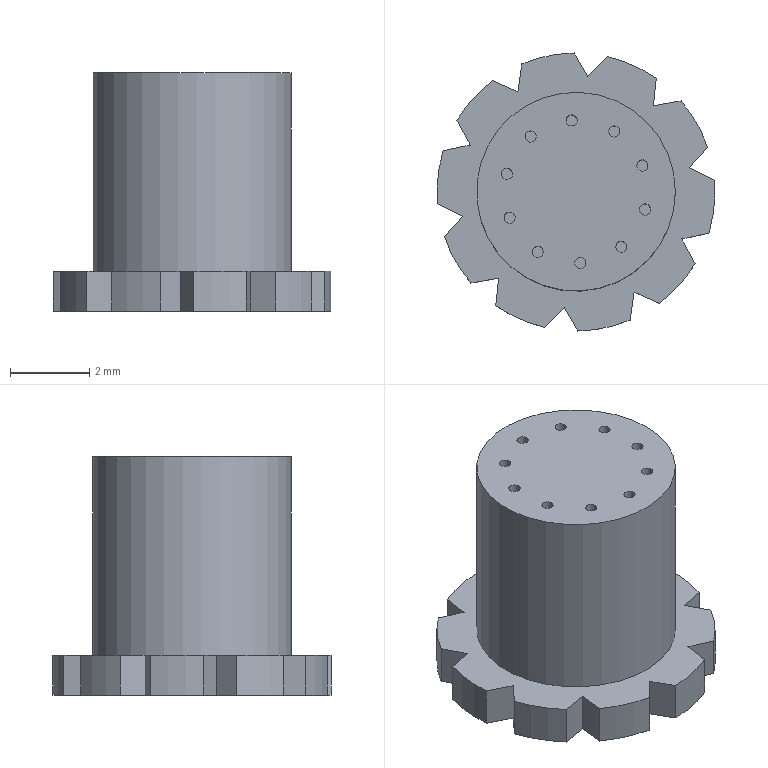Part | NX | features DATUM_CSYS 3, CYLINDER 2, EXTRUDE 2, SKETCH 2 | 1 solid | 54 faces | box 7 x 6.999 x 6 mm | volume 131.027 mm3 | plane 33 | cylinder 21 | commonest cylinder face diameters 0.283 x10 7 x10 5 x1
STEP:
#1=CARTESIAN_POINT('',(-0.7918,-3.409,0.));
#2=VERTEX_POINT('',#1);
#3=CARTESIAN_POINT('',(-0.7918,-3.409,-1.));
#4=VERTEX_POINT('',#3);
#5=CARTESIAN_POINT('',(-0.7918,-3.409,0.));
#6=DIRECTION('',(0.,0.,-1.));
#7=VECTOR('',#6,1000.);
#8=LINE('',#5,#7);
#9=EDGE_CURVE('',#2,#4,#8,.T.);
#10=ORIENTED_EDGE('',*,*,#9,.F.);
#11=CARTESIAN_POINT('',(-2.021,-2.858,0.));
#12=VERTEX_POINT('',#11);
#13=CARTESIAN_POINT('',(0.,0.,0.));
#14=DIRECTION('',(0.,0.,-1.));
#15=DIRECTION('',(1.,0.,0.));
#16=AXIS2_PLACEMENT_3D('',#13,#14,#15);
#17=CIRCLE('',#16,3.5);
#18=EDGE_CURVE('',#2,#12,#17,.T.);
#19=ORIENTED_EDGE('',*,*,#18,.T.);
#20=CARTESIAN_POINT('',(-2.021,-2.858,-1.));
#21=VERTEX_POINT('',#20);
#22=CARTESIAN_POINT('',(-2.021,-2.858,0.));
#23=DIRECTION('',(0.,0.,-1.));
#24=VECTOR('',#23,1000.);
#25=LINE('',#22,#24);
#26=EDGE_CURVE('',#21,#12,#25,.F.);
#27=ORIENTED_EDGE('',*,*,#26,.F.);
#28=CARTESIAN_POINT('',(0.,0.,-1.));
#29=DIRECTION('',(0.,0.,1.));
#30=DIRECTION('',(1.,0.,0.));
#31=AXIS2_PLACEMENT_3D('',#28,#29,#30);
#32=CIRCLE('',#31,3.5);
#33=EDGE_CURVE('',#21,#4,#32,.T.);
#34=ORIENTED_EDGE('',*,*,#33,.T.);
#35=EDGE_LOOP('',(#10,#19,#27,#34));
#36=FACE_BOUND('',#35,.T.);
#37=CARTESIAN_POINT('',(0.,0.,0.));
#38=DIRECTION('',(0.,0.,-1.));
#39=DIRECTION('',(1.,0.,0.));
#40=AXIS2_PLACEMENT_3D('',#37,#38,#39);
#41=CYLINDRICAL_SURFACE('',#40,3.5);
#42=ADVANCED_FACE('',(#36),#41,.T.);
#43=CARTESIAN_POINT('',(-2.093,2.805,-1.));
#44=VERTEX_POINT('',#43);
#45=CARTESIAN_POINT('',(-2.093,2.805,0.));
#46=VERTEX_POINT('',#45);
#47=CARTESIAN_POINT('',(-2.093,2.805,0.));
#48=DIRECTION('',(0.,0.,-1.));
#49=VECTOR('',#48,1000.);
#50=LINE('',#47,#49);
#51=EDGE_CURVE('',#44,#46,#50,.F.);
#52=ORIENTED_EDGE('',*,*,#51,.F.);
#53=CARTESIAN_POINT('',(-2.998,1.807,-1.));
#54=VERTEX_POINT('',#53);
#55=CARTESIAN_POINT('',(0.,0.,-1.));
#56=DIRECTION('',(0.,0.,1.));
#57=DIRECTION('',(1.,0.,0.));
#58=AXIS2_PLACEMENT_3D('',#55,#56,#57);
#59=CIRCLE('',#58,3.5);
#60=EDGE_CURVE('',#44,#54,#59,.T.);
#61=ORIENTED_EDGE('',*,*,#60,.T.);
#62=CARTESIAN_POINT('',(-2.998,1.807,0.));
#63=VERTEX_POINT('',#62);
#64=CARTESIAN_POINT('',(-2.998,1.807,0.));
#65=DIRECTION('',(0.,0.,-1.));
#66=VECTOR('',#65,1000.);
#67=LINE('',#64,#66);
#68=EDGE_CURVE('',#63,#54,#67,.T.);
#69=ORIENTED_EDGE('',*,*,#68,.F.);
#70=CARTESIAN_POINT('',(0.,0.,0.));
#71=DIRECTION('',(0.,0.,-1.));
#72=DIRECTION('',(1.,0.,0.));
#73=AXIS2_PLACEMENT_3D('',#70,#71,#72);
#74=CIRCLE('',#73,3.5);
#75=EDGE_CURVE('',#63,#46,#74,.T.);
#76=ORIENTED_EDGE('',*,*,#75,.T.);
#77=EDGE_LOOP('',(#52,#61,#69,#76));
#78=FACE_BOUND('',#77,.T.);
#79=CARTESIAN_POINT('',(0.,0.,0.));
#80=DIRECTION('',(0.,0.,-1.));
#81=DIRECTION('',(1.,0.,0.));
#82=AXIS2_PLACEMENT_3D('',#79,#80,#81);
#83=CYLINDRICAL_SURFACE('',#82,3.5);
#84=ADVANCED_FACE('',(#78),#83,.T.);
#85=CARTESIAN_POINT('',(0.04482,-3.5,-1.));
#86=VERTEX_POINT('',#85);
#87=CARTESIAN_POINT('',(0.04482,-3.5,0.));
#88=VERTEX_POINT('',#87);
#89=CARTESIAN_POINT('',(0.04482,-3.5,0.));
#90=DIRECTION('',(0.,0.,-1.));
#91=VECTOR('',#90,1000.);
#92=LINE('',#89,#91);
#93=EDGE_CURVE('',#86,#88,#92,.F.);
#94=ORIENTED_EDGE('',*,*,#93,.F.);
#95=CARTESIAN_POINT('',(1.363,-3.224,-1.));
#96=VERTEX_POINT('',#95);
#97=CARTESIAN_POINT('',(0.,0.,-1.));
#98=DIRECTION('',(0.,0.,1.));
#99=DIRECTION('',(1.,0.,0.));
#100=AXIS2_PLACEMENT_3D('',#97,#98,#99);
#101=CIRCLE('',#100,3.5);
#102=EDGE_CURVE('',#86,#96,#101,.T.);
#103=ORIENTED_EDGE('',*,*,#102,.T.);
#104=CARTESIAN_POINT('',(1.363,-3.224,0.));
#105=VERTEX_POINT('',#104);
#106=CARTESIAN_POINT('',(1.363,-3.224,0.));
#107=DIRECTION('',(0.,0.,-1.));
#108=VECTOR('',#107,1000.);
#109=LINE('',#106,#108);
#110=EDGE_CURVE('',#105,#96,#109,.T.);
#111=ORIENTED_EDGE('',*,*,#110,.F.);
#112=CARTESIAN_POINT('',(0.,0.,0.));
#113=DIRECTION('',(0.,0.,-1.));
#114=DIRECTION('',(1.,0.,0.));
#115=AXIS2_PLACEMENT_3D('',#112,#113,#114);
#116=CIRCLE('',#115,3.5);
#117=EDGE_CURVE('',#105,#88,#116,.T.);
#118=ORIENTED_EDGE('',*,*,#117,.T.);
#119=EDGE_LOOP('',(#94,#103,#111,#118));
#120=FACE_BOUND('',#119,.T.);
#121=CARTESIAN_POINT('',(0.,0.,0.));
#122=DIRECTION('',(0.,0.,-1.));
#123=DIRECTION('',(1.,0.,0.));
#124=AXIS2_PLACEMENT_3D('',#121,#122,#123);
#125=CYLINDRICAL_SURFACE('',#124,3.5);
#126=ADVANCED_FACE('',(#120),#125,.T.);
#127=CARTESIAN_POINT('',(-2.644,-2.293,0.));
#128=VERTEX_POINT('',#127);
#129=CARTESIAN_POINT('',(-2.644,-2.293,-1.));
#130=VERTEX_POINT('',#129);
#131=CARTESIAN_POINT('',(-2.644,-2.293,0.));
#132=DIRECTION('',(0.,0.,-1.));
#133=VECTOR('',#132,1000.);
#134=LINE('',#131,#133);
#135=EDGE_CURVE('',#128,#130,#134,.T.);
#136=ORIENTED_EDGE('',*,*,#135,.F.);
#137=CARTESIAN_POINT('',(-3.315,-1.124,0.));
#138=VERTEX_POINT('',#137);
#139=CARTESIAN_POINT('',(0.,0.,0.));
#140=DIRECTION('',(0.,0.,-1.));
#141=DIRECTION('',(1.,0.,0.));
#142=AXIS2_PLACEMENT_3D('',#139,#140,#141);
#143=CIRCLE('',#142,3.5);
#144=EDGE_CURVE('',#128,#138,#143,.T.);
#145=ORIENTED_EDGE('',*,*,#144,.T.);
#146=CARTESIAN_POINT('',(-3.315,-1.124,-1.));
#147=VERTEX_POINT('',#146);
#148=CARTESIAN_POINT('',(-3.315,-1.124,0.));
#149=DIRECTION('',(0.,0.,-1.));
#150=VECTOR('',#149,1000.);
#151=LINE('',#148,#150);
#152=EDGE_CURVE('',#147,#138,#151,.F.);
#153=ORIENTED_EDGE('',*,*,#152,.F.);
#154=CARTESIAN_POINT('',(0.,0.,-1.));
#155=DIRECTION('',(0.,0.,1.));
#156=DIRECTION('',(1.,0.,0.));
#157=AXIS2_PLACEMENT_3D('',#154,#155,#156);
#158=CIRCLE('',#157,3.5);
#159=EDGE_CURVE('',#147,#130,#158,.T.);
#160=ORIENTED_EDGE('',*,*,#159,.T.);
#161=EDGE_LOOP('',(#136,#145,#153,#160));
#162=FACE_BOUND('',#161,.T.);
#163=CARTESIAN_POINT('',(0.,0.,0.));
#164=DIRECTION('',(0.,0.,-1.));
#165=DIRECTION('',(1.,0.,0.));
#166=AXIS2_PLACEMENT_3D('',#163,#164,#165);
#167=CYLINDRICAL_SURFACE('',#166,3.5);
#168=ADVANCED_FACE('',(#162),#167,.T.);
#169=CARTESIAN_POINT('',(2.998,-1.807,0.));
#170=VERTEX_POINT('',#169);
#171=CARTESIAN_POINT('',(2.998,-1.807,-1.));
#172=VERTEX_POINT('',#171);
#173=CARTESIAN_POINT('',(2.998,-1.807,0.));
#174=DIRECTION('',(0.,0.,-1.));
#175=VECTOR('',#174,1000.);
#176=LINE('',#173,#175);
#177=EDGE_CURVE('',#170,#172,#176,.T.);
#178=ORIENTED_EDGE('',*,*,#177,.F.);
#179=CARTESIAN_POINT('',(2.093,-2.805,0.));
#180=VERTEX_POINT('',#179);
#181=CARTESIAN_POINT('',(0.,0.,0.));
#182=DIRECTION('',(0.,0.,-1.));
#183=DIRECTION('',(1.,0.,0.));
#184=AXIS2_PLACEMENT_3D('',#181,#182,#183);
#185=CIRCLE('',#184,3.5);
#186=EDGE_CURVE('',#170,#180,#185,.T.);
#187=ORIENTED_EDGE('',*,*,#186,.T.);
#188=CARTESIAN_POINT('',(2.093,-2.805,-1.));
#189=VERTEX_POINT('',#188);
#190=CARTESIAN_POINT('',(2.093,-2.805,0.));
#191=DIRECTION('',(0.,0.,-1.));
#192=VECTOR('',#191,1000.);
#193=LINE('',#190,#192);
#194=EDGE_CURVE('',#189,#180,#193,.F.);
#195=ORIENTED_EDGE('',*,*,#194,.F.);
#196=CARTESIAN_POINT('',(0.,0.,-1.));
#197=DIRECTION('',(0.,0.,1.));
#198=DIRECTION('',(1.,0.,0.));
#199=AXIS2_PLACEMENT_3D('',#196,#197,#198);
#200=CIRCLE('',#199,3.5);
#201=EDGE_CURVE('',#189,#172,#200,.T.);
#202=ORIENTED_EDGE('',*,*,#201,.T.);
#203=EDGE_LOOP('',(#178,#187,#195,#202));
#204=FACE_BOUND('',#203,.T.);
#205=CARTESIAN_POINT('',(0.,0.,0.));
#206=DIRECTION('',(0.,0.,-1.));
#207=DIRECTION('',(1.,0.,0.));
#208=AXIS2_PLACEMENT_3D('',#205,#206,#207);
#209=CYLINDRICAL_SURFACE('',#208,3.5);
#210=ADVANCED_FACE('',(#204),#209,.T.);
#211=CARTESIAN_POINT('',(2.021,2.858,-1.));
#212=VERTEX_POINT('',#211);
#213=CARTESIAN_POINT('',(2.021,2.858,0.));
#214=VERTEX_POINT('',#213);
#215=CARTESIAN_POINT('',(2.021,2.858,0.));
#216=DIRECTION('',(0.,0.,-1.));
#217=VECTOR('',#216,1000.);
#218=LINE('',#215,#217);
#219=EDGE_CURVE('',#212,#214,#218,.F.);
#220=ORIENTED_EDGE('',*,*,#219,.F.);
#221=CARTESIAN_POINT('',(0.7918,3.409,-1.));
#222=VERTEX_POINT('',#221);
#223=CARTESIAN_POINT('',(0.,0.,-1.));
#224=DIRECTION('',(0.,0.,1.));
#225=DIRECTION('',(1.,0.,0.));
#226=AXIS2_PLACEMENT_3D('',#223,#224,#225);
#227=CIRCLE('',#226,3.5);
#228=EDGE_CURVE('',#212,#222,#227,.T.);
#229=ORIENTED_EDGE('',*,*,#228,.T.);
#230=CARTESIAN_POINT('',(0.7918,3.409,0.));
#231=VERTEX_POINT('',#230);
#232=CARTESIAN_POINT('',(0.7918,3.409,0.));
#233=DIRECTION('',(0.,0.,-1.));
#234=VECTOR('',#233,1000.);
#235=LINE('',#232,#234);
#236=EDGE_CURVE('',#231,#222,#235,.T.);
#237=ORIENTED_EDGE('',*,*,#236,.F.);
#238=CARTESIAN_POINT('',(0.,0.,0.));
#239=DIRECTION('',(0.,0.,-1.));
#240=DIRECTION('',(1.,0.,0.));
#241=AXIS2_PLACEMENT_3D('',#238,#239,#240);
#242=CIRCLE('',#241,3.5);
#243=EDGE_CURVE('',#231,#214,#242,.T.);
#244=ORIENTED_EDGE('',*,*,#243,.T.);
#245=EDGE_LOOP('',(#220,#229,#237,#244));
#246=FACE_BOUND('',#245,.T.);
#247=CARTESIAN_POINT('',(0.,0.,0.));
#248=DIRECTION('',(0.,0.,-1.));
#249=DIRECTION('',(1.,0.,0.));
#250=AXIS2_PLACEMENT_3D('',#247,#248,#249);
#251=CYLINDRICAL_SURFACE('',#250,3.5);
#252=ADVANCED_FACE('',(#246),#251,.T.);
#253=CARTESIAN_POINT('',(-3.487,-0.3005,0.));
#254=VERTEX_POINT('',#253);
#255=CARTESIAN_POINT('',(-3.487,-0.3005,-1.));
#256=VERTEX_POINT('',#255);
#257=CARTESIAN_POINT('',(-3.487,-0.3005,0.));
#258=DIRECTION('',(0.,0.,-1.));
#259=VECTOR('',#258,1000.);
#260=LINE('',#257,#259);
#261=EDGE_CURVE('',#254,#256,#260,.T.);
#262=ORIENTED_EDGE('',*,*,#261,.F.);
#263=CARTESIAN_POINT('',(-3.342,1.039,0.));
#264=VERTEX_POINT('',#263);
#265=CARTESIAN_POINT('',(0.,0.,0.));
#266=DIRECTION('',(0.,0.,-1.));
#267=DIRECTION('',(1.,0.,0.));
#268=AXIS2_PLACEMENT_3D('',#265,#266,#267);
#269=CIRCLE('',#268,3.5);
#270=EDGE_CURVE('',#254,#264,#269,.T.);
#271=ORIENTED_EDGE('',*,*,#270,.T.);
#272=CARTESIAN_POINT('',(-3.342,1.039,-1.));
#273=VERTEX_POINT('',#272);
#274=CARTESIAN_POINT('',(-3.342,1.039,0.));
#275=DIRECTION('',(0.,0.,-1.));
#276=VECTOR('',#275,1000.);
#277=LINE('',#274,#276);
#278=EDGE_CURVE('',#273,#264,#277,.F.);
#279=ORIENTED_EDGE('',*,*,#278,.F.);
#280=CARTESIAN_POINT('',(0.,0.,-1.));
#281=DIRECTION('',(0.,0.,1.));
#282=DIRECTION('',(1.,0.,0.));
#283=AXIS2_PLACEMENT_3D('',#280,#281,#282);
#284=CIRCLE('',#283,3.5);
#285=EDGE_CURVE('',#273,#256,#284,.T.);
#286=ORIENTED_EDGE('',*,*,#285,.T.);
#287=EDGE_LOOP('',(#262,#271,#279,#286));
#288=FACE_BOUND('',#287,.T.);
#289=CARTESIAN_POINT('',(0.,0.,0.));
#290=DIRECTION('',(0.,0.,-1.));
#291=DIRECTION('',(1.,0.,0.));
#292=AXIS2_PLACEMENT_3D('',#289,#290,#291);
#293=CYLINDRICAL_SURFACE('',#292,3.5);
#294=ADVANCED_FACE('',(#288),#293,.T.);
#295=CARTESIAN_POINT('',(-1.363,3.224,0.));
#296=VERTEX_POINT('',#295);
#297=CARTESIAN_POINT('',(-1.363,3.224,-1.));
#298=VERTEX_POINT('',#297);
#299=CARTESIAN_POINT('',(-1.363,3.224,0.));
#300=DIRECTION('',(0.,0.,-1.));
#301=VECTOR('',#300,1000.);
#302=LINE('',#299,#301);
#303=EDGE_CURVE('',#296,#298,#302,.T.);
#304=ORIENTED_EDGE('',*,*,#303,.F.);
#305=CARTESIAN_POINT('',(-0.04482,3.5,0.));
#306=VERTEX_POINT('',#305);
#307=CARTESIAN_POINT('',(0.,0.,0.));
#308=DIRECTION('',(0.,0.,-1.));
#309=DIRECTION('',(1.,0.,0.));
#310=AXIS2_PLACEMENT_3D('',#307,#308,#309);
#311=CIRCLE('',#310,3.5);
#312=EDGE_CURVE('',#296,#306,#311,.T.);
#313=ORIENTED_EDGE('',*,*,#312,.T.);
#314=CARTESIAN_POINT('',(-0.04482,3.5,-1.));
#315=VERTEX_POINT('',#314);
#316=CARTESIAN_POINT('',(-0.04482,3.5,0.));
#317=DIRECTION('',(0.,0.,-1.));
#318=VECTOR('',#317,1000.);
#319=LINE('',#316,#318);
#320=EDGE_CURVE('',#315,#306,#319,.F.);
#321=ORIENTED_EDGE('',*,*,#320,.F.);
#322=CARTESIAN_POINT('',(0.,0.,-1.));
#323=DIRECTION('',(0.,0.,1.));
#324=DIRECTION('',(1.,0.,0.));
#325=AXIS2_PLACEMENT_3D('',#322,#323,#324);
#326=CIRCLE('',#325,3.5);
#327=EDGE_CURVE('',#315,#298,#326,.T.);
#328=ORIENTED_EDGE('',*,*,#327,.T.);
#329=EDGE_LOOP('',(#304,#313,#321,#328));
#330=FACE_BOUND('',#329,.T.);
#331=CARTESIAN_POINT('',(0.,0.,0.));
#332=DIRECTION('',(0.,0.,-1.));
#333=DIRECTION('',(1.,0.,0.));
#334=AXIS2_PLACEMENT_3D('',#331,#332,#333);
#335=CYLINDRICAL_SURFACE('',#334,3.5);
#336=ADVANCED_FACE('',(#330),#335,.T.);
#337=CARTESIAN_POINT('',(3.342,-1.039,-1.));
#338=VERTEX_POINT('',#337);
#339=CARTESIAN_POINT('',(3.342,-1.039,0.));
#340=VERTEX_POINT('',#339);
#341=CARTESIAN_POINT('',(3.342,-1.039,0.));
#342=DIRECTION('',(0.,0.,-1.));
#343=VECTOR('',#342,1000.);
#344=LINE('',#341,#343);
#345=EDGE_CURVE('',#338,#340,#344,.F.);
#346=ORIENTED_EDGE('',*,*,#345,.F.);
#347=CARTESIAN_POINT('',(3.487,0.3005,-1.));
#348=VERTEX_POINT('',#347);
#349=CARTESIAN_POINT('',(0.,0.,-1.));
#350=DIRECTION('',(0.,0.,1.));
#351=DIRECTION('',(1.,0.,0.));
#352=AXIS2_PLACEMENT_3D('',#349,#350,#351);
#353=CIRCLE('',#352,3.5);
#354=EDGE_CURVE('',#338,#348,#353,.T.);
#355=ORIENTED_EDGE('',*,*,#354,.T.);
#356=CARTESIAN_POINT('',(3.487,0.3005,0.));
#357=VERTEX_POINT('',#356);
#358=CARTESIAN_POINT('',(3.487,0.3005,0.));
#359=DIRECTION('',(0.,0.,-1.));
#360=VECTOR('',#359,1000.);
#361=LINE('',#358,#360);
#362=EDGE_CURVE('',#357,#348,#361,.T.);
#363=ORIENTED_EDGE('',*,*,#362,.F.);
#364=CARTESIAN_POINT('',(0.,0.,0.));
#365=DIRECTION('',(0.,0.,-1.));
#366=DIRECTION('',(1.,0.,0.));
#367=AXIS2_PLACEMENT_3D('',#364,#365,#366);
#368=CIRCLE('',#367,3.5);
#369=EDGE_CURVE('',#357,#340,#368,.T.);
#370=ORIENTED_EDGE('',*,*,#369,.T.);
#371=EDGE_LOOP('',(#346,#355,#363,#370));
#372=FACE_BOUND('',#371,.T.);
#373=CARTESIAN_POINT('',(0.,0.,0.));
#374=DIRECTION('',(0.,0.,-1.));
#375=DIRECTION('',(1.,0.,0.));
#376=AXIS2_PLACEMENT_3D('',#373,#374,#375);
#377=CYLINDRICAL_SURFACE('',#376,3.5);
#378=ADVANCED_FACE('',(#372),#377,.T.);
#379=CARTESIAN_POINT('',(0.03282,1.793,5.));
#380=VERTEX_POINT('',#379);
#381=CARTESIAN_POINT('',(-0.1085,1.793,5.));
#382=DIRECTION('',(0.,0.,1.));
#383=DIRECTION('',(1.,0.,0.));
#384=AXIS2_PLACEMENT_3D('',#381,#382,#383);
#385=CIRCLE('',#384,0.1413);
#386=EDGE_CURVE('',#380,#380,#385,.T.);
#387=ORIENTED_EDGE('',*,*,#386,.F.);
#388=EDGE_LOOP('',(#387));
#389=FACE_BOUND('',#388,.T.);
#390=CARTESIAN_POINT('',(-1.08,-1.431,5.));
#391=VERTEX_POINT('',#390);
#392=CARTESIAN_POINT('',(-0.9659,-1.514,5.));
#393=DIRECTION('',(0.,0.,1.));
#394=DIRECTION('',(-0.809,0.5878,0.));
#395=AXIS2_PLACEMENT_3D('',#392,#393,#394);
#396=CIRCLE('',#395,0.1413);
#397=EDGE_CURVE('',#391,#391,#396,.T.);
#398=ORIENTED_EDGE('',*,*,#397,.F.);
#399=EDGE_LOOP('',(#398));
#400=FACE_BOUND('',#399,.T.);
#401=CARTESIAN_POINT('',(-1.027,1.47,5.));
#402=VERTEX_POINT('',#401);
#403=CARTESIAN_POINT('',(-1.141,1.386,5.));
#404=DIRECTION('',(0.,0.,1.));
#405=DIRECTION('',(0.809,0.5878,0.));
#406=AXIS2_PLACEMENT_3D('',#403,#404,#405);
#407=CIRCLE('',#406,0.1413);
#408=EDGE_CURVE('',#402,#402,#407,.T.);
#409=ORIENTED_EDGE('',*,*,#408,.F.);
#410=EDGE_LOOP('',(#409));
#411=FACE_BOUND('',#410,.T.);
#412=CARTESIAN_POINT('',(-1.715,-0.5227,5.));
#413=VERTEX_POINT('',#412);
#414=CARTESIAN_POINT('',(-1.671,-0.6571,5.));
#415=DIRECTION('',(0.,0.,1.));
#416=DIRECTION('',(-0.309,0.9511,0.));
#417=AXIS2_PLACEMENT_3D('',#414,#415,#416);
#418=CIRCLE('',#417,0.1413);
#419=EDGE_CURVE('',#413,#413,#418,.T.);
#420=ORIENTED_EDGE('',*,*,#419,.F.);
#421=EDGE_LOOP('',(#420));
#422=FACE_BOUND('',#421,.T.);
#423=CARTESIAN_POINT('',(1.715,0.5227,5.));
#424=VERTEX_POINT('',#423);
#425=CARTESIAN_POINT('',(1.671,0.6571,5.));
#426=DIRECTION('',(0.,0.,1.));
#427=DIRECTION('',(0.309,-0.9511,0.));
#428=AXIS2_PLACEMENT_3D('',#425,#426,#427);
#429=CIRCLE('',#428,0.1413);
#430=EDGE_CURVE('',#424,#424,#429,.T.);
#431=ORIENTED_EDGE('',*,*,#430,.F.);
#432=EDGE_LOOP('',(#431));
#433=FACE_BOUND('',#432,.T.);
#434=CARTESIAN_POINT('',(1.027,-1.47,5.));
#435=VERTEX_POINT('',#434);
#436=CARTESIAN_POINT('',(1.141,-1.386,5.));
#437=DIRECTION('',(0.,0.,1.));
#438=DIRECTION('',(-0.809,-0.5878,0.));
#439=AXIS2_PLACEMENT_3D('',#436,#437,#438);
#440=CIRCLE('',#439,0.1413);
#441=EDGE_CURVE('',#435,#435,#440,.T.);
#442=ORIENTED_EDGE('',*,*,#441,.F.);
#443=EDGE_LOOP('',(#442));
#444=FACE_BOUND('',#443,.T.);
#445=CARTESIAN_POINT('',(1.08,1.431,5.));
#446=VERTEX_POINT('',#445);
#447=CARTESIAN_POINT('',(0.9659,1.514,5.));
#448=DIRECTION('',(0.,0.,1.));
#449=DIRECTION('',(0.809,-0.5878,0.));
#450=AXIS2_PLACEMENT_3D('',#447,#448,#449);
#451=CIRCLE('',#450,0.1413);
#452=EDGE_CURVE('',#446,#446,#451,.T.);
#453=ORIENTED_EDGE('',*,*,#452,.F.);
#454=EDGE_LOOP('',(#453));
#455=FACE_BOUND('',#454,.T.);
#456=CARTESIAN_POINT('',(-0.03282,-1.793,5.));
#457=VERTEX_POINT('',#456);
#458=CARTESIAN_POINT('',(0.1085,-1.793,5.));
#459=DIRECTION('',(0.,0.,1.));
#460=DIRECTION('',(-1.,0.,0.));
#461=AXIS2_PLACEMENT_3D('',#458,#459,#460);
#462=CIRCLE('',#461,0.1413);
#463=EDGE_CURVE('',#457,#457,#462,.T.);
#464=ORIENTED_EDGE('',*,*,#463,.F.);
#465=EDGE_LOOP('',(#464));
#466=FACE_BOUND('',#465,.T.);
#467=CARTESIAN_POINT('',(-1.695,0.5852,5.));
#468=VERTEX_POINT('',#467);
#469=CARTESIAN_POINT('',(-1.738,0.4508,5.));
#470=DIRECTION('',(0.,0.,1.));
#471=DIRECTION('',(0.309,0.9511,0.));
#472=AXIS2_PLACEMENT_3D('',#469,#470,#471);
#473=CIRCLE('',#472,0.1413);
#474=EDGE_CURVE('',#468,#468,#473,.T.);
#475=ORIENTED_EDGE('',*,*,#474,.F.);
#476=EDGE_LOOP('',(#475));
#477=FACE_BOUND('',#476,.T.);
#478=CARTESIAN_POINT('',(1.695,-0.5852,5.));
#479=VERTEX_POINT('',#478);
#480=CARTESIAN_POINT('',(1.738,-0.4508,5.));
#481=DIRECTION('',(0.,0.,1.));
#482=DIRECTION('',(-0.309,-0.9511,0.));
#483=AXIS2_PLACEMENT_3D('',#480,#481,#482);
#484=CIRCLE('',#483,0.1413);
#485=EDGE_CURVE('',#479,#479,#484,.T.);
#486=ORIENTED_EDGE('',*,*,#485,.F.);
#487=EDGE_LOOP('',(#486));
#488=FACE_BOUND('',#487,.T.);
#489=CARTESIAN_POINT('',(2.5,0.,5.));
#490=VERTEX_POINT('',#489);
#491=CARTESIAN_POINT('',(0.,0.,5.));
#492=DIRECTION('',(0.,0.,-1.));
#493=DIRECTION('',(1.,0.,0.));
#494=AXIS2_PLACEMENT_3D('',#491,#492,#493);
#495=CIRCLE('',#494,2.5);
#496=EDGE_CURVE('',#490,#490,#495,.T.);
#497=ORIENTED_EDGE('',*,*,#496,.F.);
#498=EDGE_LOOP('',(#497));
#499=FACE_BOUND('',#498,.T.);
#500=CARTESIAN_POINT('',(0.,0.,5.));
#501=DIRECTION('',(0.,0.,1.));
#502=DIRECTION('',(1.,0.,0.));
#503=AXIS2_PLACEMENT_3D('',#500,#501,#502);
#504=PLANE('',#503);
#505=ADVANCED_FACE('',(#389,#400,#411,#422,#433,#444,#455,#466,#477,#488,#499),#504,.T.);
#506=ORIENTED_EDGE('',*,*,#496,.T.);
#507=EDGE_LOOP('',(#506));
#508=FACE_BOUND('',#507,.T.);
#509=CARTESIAN_POINT('',(2.5,0.,0.));
#510=VERTEX_POINT('',#509);
#511=CARTESIAN_POINT('',(0.,0.,0.));
#512=DIRECTION('',(0.,0.,1.));
#513=DIRECTION('',(1.,0.,0.));
#514=AXIS2_PLACEMENT_3D('',#511,#512,#513);
#515=CIRCLE('',#514,2.5);
#516=EDGE_CURVE('',#510,#510,#515,.T.);
#517=ORIENTED_EDGE('',*,*,#516,.T.);
#518=EDGE_LOOP('',(#517));
#519=FACE_BOUND('',#518,.T.);
#520=CARTESIAN_POINT('',(0.,0.,0.));
#521=DIRECTION('',(0.,0.,1.));
#522=DIRECTION('',(1.,0.,0.));
#523=AXIS2_PLACEMENT_3D('',#520,#521,#522);
#524=CYLINDRICAL_SURFACE('',#523,2.5);
#525=ADVANCED_FACE('',(#508,#519),#524,.T.);
#526=ORIENTED_EDGE('',*,*,#485,.T.);
#527=EDGE_LOOP('',(#526));
#528=FACE_BOUND('',#527,.T.);
#529=CARTESIAN_POINT('',(1.695,-0.5852,0.));
#530=VERTEX_POINT('',#529);
#531=CARTESIAN_POINT('',(1.738,-0.4508,0.));
#532=DIRECTION('',(0.,0.,1.));
#533=DIRECTION('',(-0.309,-0.9511,0.));
#534=AXIS2_PLACEMENT_3D('',#531,#532,#533);
#535=CIRCLE('',#534,0.1413);
#536=EDGE_CURVE('',#530,#530,#535,.T.);
#537=ORIENTED_EDGE('',*,*,#536,.F.);
#538=EDGE_LOOP('',(#537));
#539=FACE_BOUND('',#538,.T.);
#540=CARTESIAN_POINT('',(1.738,-0.4508,5.));
#541=DIRECTION('',(0.,0.,-1.));
#542=DIRECTION('',(-1.,0.,0.));
#543=AXIS2_PLACEMENT_3D('',#540,#541,#542);
#544=CYLINDRICAL_SURFACE('',#543,0.1413);
#545=ADVANCED_FACE('',(#528,#539),#544,.F.);
#546=ORIENTED_EDGE('',*,*,#474,.T.);
#547=EDGE_LOOP('',(#546));
#548=FACE_BOUND('',#547,.T.);
#549=CARTESIAN_POINT('',(-1.695,0.5852,0.));
#550=VERTEX_POINT('',#549);
#551=CARTESIAN_POINT('',(-1.738,0.4508,0.));
#552=DIRECTION('',(0.,0.,1.));
#553=DIRECTION('',(0.309,0.9511,0.));
#554=AXIS2_PLACEMENT_3D('',#551,#552,#553);
#555=CIRCLE('',#554,0.1413);
#556=EDGE_CURVE('',#550,#550,#555,.T.);
#557=ORIENTED_EDGE('',*,*,#556,.F.);
#558=EDGE_LOOP('',(#557));
#559=FACE_BOUND('',#558,.T.);
#560=CARTESIAN_POINT('',(-1.738,0.4508,5.));
#561=DIRECTION('',(0.,0.,-1.));
#562=DIRECTION('',(-1.,0.,0.));
#563=AXIS2_PLACEMENT_3D('',#560,#561,#562);
#564=CYLINDRICAL_SURFACE('',#563,0.1413);
#565=ADVANCED_FACE('',(#548,#559),#564,.F.);
#566=ORIENTED_EDGE('',*,*,#463,.T.);
#567=EDGE_LOOP('',(#566));
#568=FACE_BOUND('',#567,.T.);
#569=CARTESIAN_POINT('',(-0.03282,-1.793,0.));
#570=VERTEX_POINT('',#569);
#571=CARTESIAN_POINT('',(0.1085,-1.793,0.));
#572=DIRECTION('',(0.,0.,1.));
#573=DIRECTION('',(-1.,0.,0.));
#574=AXIS2_PLACEMENT_3D('',#571,#572,#573);
#575=CIRCLE('',#574,0.1413);
#576=EDGE_CURVE('',#570,#570,#575,.T.);
#577=ORIENTED_EDGE('',*,*,#576,.F.);
#578=EDGE_LOOP('',(#577));
#579=FACE_BOUND('',#578,.T.);
#580=CARTESIAN_POINT('',(0.1085,-1.793,5.));
#581=DIRECTION('',(0.,0.,-1.));
#582=DIRECTION('',(-1.,0.,0.));
#583=AXIS2_PLACEMENT_3D('',#580,#581,#582);
#584=CYLINDRICAL_SURFACE('',#583,0.1413);
#585=ADVANCED_FACE('',(#568,#579),#584,.F.);
#586=ORIENTED_EDGE('',*,*,#452,.T.);
#587=EDGE_LOOP('',(#586));
#588=FACE_BOUND('',#587,.T.);
#589=CARTESIAN_POINT('',(1.08,1.431,0.));
#590=VERTEX_POINT('',#589);
#591=CARTESIAN_POINT('',(0.9659,1.514,0.));
#592=DIRECTION('',(0.,0.,1.));
#593=DIRECTION('',(0.809,-0.5878,0.));
#594=AXIS2_PLACEMENT_3D('',#591,#592,#593);
#595=CIRCLE('',#594,0.1413);
#596=EDGE_CURVE('',#590,#590,#595,.T.);
#597=ORIENTED_EDGE('',*,*,#596,.F.);
#598=EDGE_LOOP('',(#597));
#599=FACE_BOUND('',#598,.T.);
#600=CARTESIAN_POINT('',(0.9659,1.514,5.));
#601=DIRECTION('',(0.,0.,-1.));
#602=DIRECTION('',(-1.,0.,0.));
#603=AXIS2_PLACEMENT_3D('',#600,#601,#602);
#604=CYLINDRICAL_SURFACE('',#603,0.1413);
#605=ADVANCED_FACE('',(#588,#599),#604,.F.);
#606=ORIENTED_EDGE('',*,*,#441,.T.);
#607=EDGE_LOOP('',(#606));
#608=FACE_BOUND('',#607,.T.);
#609=CARTESIAN_POINT('',(1.027,-1.47,0.));
#610=VERTEX_POINT('',#609);
#611=CARTESIAN_POINT('',(1.141,-1.386,0.));
#612=DIRECTION('',(0.,0.,1.));
#613=DIRECTION('',(-0.809,-0.5878,0.));
#614=AXIS2_PLACEMENT_3D('',#611,#612,#613);
#615=CIRCLE('',#614,0.1413);
#616=EDGE_CURVE('',#610,#610,#615,.T.);
#617=ORIENTED_EDGE('',*,*,#616,.F.);
#618=EDGE_LOOP('',(#617));
#619=FACE_BOUND('',#618,.T.);
#620=CARTESIAN_POINT('',(1.141,-1.386,5.));
#621=DIRECTION('',(0.,0.,-1.));
#622=DIRECTION('',(-1.,0.,0.));
#623=AXIS2_PLACEMENT_3D('',#620,#621,#622);
#624=CYLINDRICAL_SURFACE('',#623,0.1413);
#625=ADVANCED_FACE('',(#608,#619),#624,.F.);
#626=ORIENTED_EDGE('',*,*,#430,.T.);
#627=EDGE_LOOP('',(#626));
#628=FACE_BOUND('',#627,.T.);
#629=CARTESIAN_POINT('',(1.715,0.5227,0.));
#630=VERTEX_POINT('',#629);
#631=CARTESIAN_POINT('',(1.671,0.6571,0.));
#632=DIRECTION('',(0.,0.,1.));
#633=DIRECTION('',(0.309,-0.9511,0.));
#634=AXIS2_PLACEMENT_3D('',#631,#632,#633);
#635=CIRCLE('',#634,0.1413);
#636=EDGE_CURVE('',#630,#630,#635,.T.);
#637=ORIENTED_EDGE('',*,*,#636,.F.);
#638=EDGE_LOOP('',(#637));
#639=FACE_BOUND('',#638,.T.);
#640=CARTESIAN_POINT('',(1.671,0.6571,5.));
#641=DIRECTION('',(0.,0.,-1.));
#642=DIRECTION('',(-1.,0.,0.));
#643=AXIS2_PLACEMENT_3D('',#640,#641,#642);
#644=CYLINDRICAL_SURFACE('',#643,0.1413);
#645=ADVANCED_FACE('',(#628,#639),#644,.F.);
#646=ORIENTED_EDGE('',*,*,#419,.T.);
#647=EDGE_LOOP('',(#646));
#648=FACE_BOUND('',#647,.T.);
#649=CARTESIAN_POINT('',(-1.715,-0.5227,0.));
#650=VERTEX_POINT('',#649);
#651=CARTESIAN_POINT('',(-1.671,-0.6571,0.));
#652=DIRECTION('',(0.,0.,1.));
#653=DIRECTION('',(-0.309,0.9511,0.));
#654=AXIS2_PLACEMENT_3D('',#651,#652,#653);
#655=CIRCLE('',#654,0.1413);
#656=EDGE_CURVE('',#650,#650,#655,.T.);
#657=ORIENTED_EDGE('',*,*,#656,.F.);
#658=EDGE_LOOP('',(#657));
#659=FACE_BOUND('',#658,.T.);
#660=CARTESIAN_POINT('',(-1.671,-0.6571,5.));
#661=DIRECTION('',(0.,0.,-1.));
#662=DIRECTION('',(-1.,0.,0.));
#663=AXIS2_PLACEMENT_3D('',#660,#661,#662);
#664=CYLINDRICAL_SURFACE('',#663,0.1413);
#665=ADVANCED_FACE('',(#648,#659),#664,.F.);
#666=ORIENTED_EDGE('',*,*,#408,.T.);
#667=EDGE_LOOP('',(#666));
#668=FACE_BOUND('',#667,.T.);
#669=CARTESIAN_POINT('',(-1.027,1.47,0.));
#670=VERTEX_POINT('',#669);
#671=CARTESIAN_POINT('',(-1.141,1.386,0.));
#672=DIRECTION('',(0.,0.,1.));
#673=DIRECTION('',(0.809,0.5878,0.));
#674=AXIS2_PLACEMENT_3D('',#671,#672,#673);
#675=CIRCLE('',#674,0.1413);
#676=EDGE_CURVE('',#670,#670,#675,.T.);
#677=ORIENTED_EDGE('',*,*,#676,.F.);
#678=EDGE_LOOP('',(#677));
#679=FACE_BOUND('',#678,.T.);
#680=CARTESIAN_POINT('',(-1.141,1.386,5.));
#681=DIRECTION('',(0.,0.,-1.));
#682=DIRECTION('',(-1.,0.,0.));
#683=AXIS2_PLACEMENT_3D('',#680,#681,#682);
#684=CYLINDRICAL_SURFACE('',#683,0.1413);
#685=ADVANCED_FACE('',(#668,#679),#684,.F.);
#686=ORIENTED_EDGE('',*,*,#397,.T.);
#687=EDGE_LOOP('',(#686));
#688=FACE_BOUND('',#687,.T.);
#689=CARTESIAN_POINT('',(-1.08,-1.431,0.));
#690=VERTEX_POINT('',#689);
#691=CARTESIAN_POINT('',(-0.9659,-1.514,0.));
#692=DIRECTION('',(0.,0.,1.));
#693=DIRECTION('',(-0.809,0.5878,0.));
#694=AXIS2_PLACEMENT_3D('',#691,#692,#693);
#695=CIRCLE('',#694,0.1413);
#696=EDGE_CURVE('',#690,#690,#695,.T.);
#697=ORIENTED_EDGE('',*,*,#696,.F.);
#698=EDGE_LOOP('',(#697));
#699=FACE_BOUND('',#698,.T.);
#700=CARTESIAN_POINT('',(-0.9659,-1.514,5.));
#701=DIRECTION('',(0.,0.,-1.));
#702=DIRECTION('',(-1.,0.,0.));
#703=AXIS2_PLACEMENT_3D('',#700,#701,#702);
#704=CYLINDRICAL_SURFACE('',#703,0.1413);
#705=ADVANCED_FACE('',(#688,#699),#704,.F.);
#706=ORIENTED_EDGE('',*,*,#386,.T.);
#707=EDGE_LOOP('',(#706));
#708=FACE_BOUND('',#707,.T.);
#709=CARTESIAN_POINT('',(0.03282,1.793,0.));
#710=VERTEX_POINT('',#709);
#711=CARTESIAN_POINT('',(-0.1085,1.793,0.));
#712=DIRECTION('',(0.,0.,1.));
#713=DIRECTION('',(1.,0.,0.));
#714=AXIS2_PLACEMENT_3D('',#711,#712,#713);
#715=CIRCLE('',#714,0.1413);
#716=EDGE_CURVE('',#710,#710,#715,.T.);
#717=ORIENTED_EDGE('',*,*,#716,.F.);
#718=EDGE_LOOP('',(#717));
#719=FACE_BOUND('',#718,.T.);
#720=CARTESIAN_POINT('',(-0.1085,1.793,5.));
#721=DIRECTION('',(0.,0.,-1.));
#722=DIRECTION('',(-1.,0.,0.));
#723=AXIS2_PLACEMENT_3D('',#720,#721,#722);
#724=CYLINDRICAL_SURFACE('',#723,0.1413);
#725=ADVANCED_FACE('',(#708,#719),#724,.F.);
#726=CARTESIAN_POINT('',(2.644,2.293,0.));
#727=VERTEX_POINT('',#726);
#728=CARTESIAN_POINT('',(2.644,2.293,-1.));
#729=VERTEX_POINT('',#728);
#730=CARTESIAN_POINT('',(2.644,2.293,0.));
#731=DIRECTION('',(0.,0.,-1.));
#732=VECTOR('',#731,1000.);
#733=LINE('',#730,#732);
#734=EDGE_CURVE('',#727,#729,#733,.T.);
#735=ORIENTED_EDGE('',*,*,#734,.F.);
#736=CARTESIAN_POINT('',(3.315,1.124,0.));
#737=VERTEX_POINT('',#736);
#738=CARTESIAN_POINT('',(0.,0.,0.));
#739=DIRECTION('',(0.,0.,-1.));
#740=DIRECTION('',(1.,0.,0.));
#741=AXIS2_PLACEMENT_3D('',#738,#739,#740);
#742=CIRCLE('',#741,3.5);
#743=EDGE_CURVE('',#727,#737,#742,.T.);
#744=ORIENTED_EDGE('',*,*,#743,.T.);
#745=CARTESIAN_POINT('',(3.315,1.124,-1.));
#746=VERTEX_POINT('',#745);
#747=CARTESIAN_POINT('',(3.315,1.124,0.));
#748=DIRECTION('',(0.,0.,-1.));
#749=VECTOR('',#748,1000.);
#750=LINE('',#747,#749);
#751=EDGE_CURVE('',#746,#737,#750,.F.);
#752=ORIENTED_EDGE('',*,*,#751,.F.);
#753=CARTESIAN_POINT('',(0.,0.,-1.));
#754=DIRECTION('',(0.,0.,1.));
#755=DIRECTION('',(1.,0.,0.));
#756=AXIS2_PLACEMENT_3D('',#753,#754,#755);
#757=CIRCLE('',#756,3.5);
#758=EDGE_CURVE('',#746,#729,#757,.T.);
#759=ORIENTED_EDGE('',*,*,#758,.T.);
#760=EDGE_LOOP('',(#735,#744,#752,#759));
#761=FACE_BOUND('',#760,.T.);
#762=CARTESIAN_POINT('',(0.,0.,0.));
#763=DIRECTION('',(0.,0.,-1.));
#764=DIRECTION('',(1.,0.,0.));
#765=AXIS2_PLACEMENT_3D('',#762,#763,#764);
#766=CYLINDRICAL_SURFACE('',#765,3.5);
#767=ADVANCED_FACE('',(#761),#766,.T.);
#768=CARTESIAN_POINT('',(-0.3,-2.9,0.));
#769=VERTEX_POINT('',#768);
#770=CARTESIAN_POINT('',(-0.3,-2.9,0.));
#771=DIRECTION('',(-0.6947,-0.7193,0.));
#772=VECTOR('',#771,1000.);
#773=LINE('',#770,#772);
#774=EDGE_CURVE('',#769,#2,#773,.T.);
#775=ORIENTED_EDGE('',*,*,#774,.F.);
#776=CARTESIAN_POINT('',(0.4189,-4.15,0.));
#777=DIRECTION('',(-0.4985,0.8669,0.));
#778=VECTOR('',#777,1000.);
#779=LINE('',#776,#778);
#780=EDGE_CURVE('',#88,#769,#779,.T.);
#781=ORIENTED_EDGE('',*,*,#780,.F.);
#782=ORIENTED_EDGE('',*,*,#117,.F.);
#783=CARTESIAN_POINT('',(1.462,-2.522,0.));
#784=VERTEX_POINT('',#783);
#785=CARTESIAN_POINT('',(1.462,-2.522,0.));
#786=DIRECTION('',(-0.1392,-0.9903,0.));
#787=VECTOR('',#786,1000.);
#788=LINE('',#785,#787);
#789=EDGE_CURVE('',#784,#105,#788,.T.);
#790=ORIENTED_EDGE('',*,*,#789,.F.);
#791=CARTESIAN_POINT('',(2.778,-3.111,0.));
#792=DIRECTION('',(-0.9128,0.4084,0.));
#793=VECTOR('',#792,1000.);
#794=LINE('',#791,#793);
#795=EDGE_CURVE('',#180,#784,#794,.T.);
#796=ORIENTED_EDGE('',*,*,#795,.F.);
#797=ORIENTED_EDGE('',*,*,#186,.F.);
#798=CARTESIAN_POINT('',(2.665,-1.181,0.));
#799=VERTEX_POINT('',#798);
#800=CARTESIAN_POINT('',(2.665,-1.181,0.));
#801=DIRECTION('',(0.4695,-0.8829,0.));
#802=VECTOR('',#801,1000.);
#803=LINE('',#800,#802);
#804=EDGE_CURVE('',#799,#170,#803,.T.);
#805=ORIENTED_EDGE('',*,*,#804,.F.);
#806=CARTESIAN_POINT('',(4.077,-0.8841,0.));
#807=DIRECTION('',(-0.9785,-0.2062,0.));
#808=VECTOR('',#807,1000.);
#809=LINE('',#806,#808);
#810=EDGE_CURVE('',#340,#799,#809,.T.);
#811=ORIENTED_EDGE('',*,*,#810,.F.);
#812=ORIENTED_EDGE('',*,*,#369,.F.);
#813=CARTESIAN_POINT('',(2.851,0.6108,0.));
#814=VERTEX_POINT('',#813);
#815=CARTESIAN_POINT('',(2.851,0.6108,0.));
#816=DIRECTION('',(0.8988,-0.4384,0.));
#817=VECTOR('',#816,1000.);
#818=LINE('',#815,#817);
#819=EDGE_CURVE('',#814,#357,#818,.T.);
#820=ORIENTED_EDGE('',*,*,#819,.F.);
#821=CARTESIAN_POINT('',(3.818,1.681,0.));
#822=DIRECTION('',(-0.6705,-0.742,0.));
#823=VECTOR('',#822,1000.);
#824=LINE('',#821,#823);
#825=EDGE_CURVE('',#737,#814,#824,.T.);
#826=ORIENTED_EDGE('',*,*,#825,.F.);
#827=ORIENTED_EDGE('',*,*,#743,.F.);
#828=CARTESIAN_POINT('',(1.947,2.17,0.));
#829=VERTEX_POINT('',#828);
#830=CARTESIAN_POINT('',(1.947,2.17,0.));
#831=DIRECTION('',(0.9848,0.1736,0.));
#832=VECTOR('',#831,1000.);
#833=LINE('',#830,#832);
#834=EDGE_CURVE('',#829,#727,#833,.T.);
#835=ORIENTED_EDGE('',*,*,#834,.F.);
#836=CARTESIAN_POINT('',(2.101,3.604,0.));
#837=DIRECTION('',(-0.1063,-0.9943,0.));
#838=VECTOR('',#837,1000.);
#839=LINE('',#836,#838);
#840=EDGE_CURVE('',#214,#829,#839,.T.);
#841=ORIENTED_EDGE('',*,*,#840,.F.);
#842=ORIENTED_EDGE('',*,*,#243,.F.);
#843=CARTESIAN_POINT('',(0.3,2.9,0.));
#844=VERTEX_POINT('',#843);
#845=CARTESIAN_POINT('',(0.3,2.9,0.));
#846=DIRECTION('',(0.6947,0.7193,0.));
#847=VECTOR('',#846,1000.);
#848=LINE('',#845,#847);
#849=EDGE_CURVE('',#844,#231,#848,.T.);
#850=ORIENTED_EDGE('',*,*,#849,.F.);
#851=CARTESIAN_POINT('',(-0.4189,4.15,0.));
#852=DIRECTION('',(0.4985,-0.8669,0.));
#853=VECTOR('',#852,1000.);
#854=LINE('',#851,#853);
#855=EDGE_CURVE('',#306,#844,#854,.T.);
#856=ORIENTED_EDGE('',*,*,#855,.F.);
#857=ORIENTED_EDGE('',*,*,#312,.F.);
#858=CARTESIAN_POINT('',(-1.462,2.522,0.));
#859=VERTEX_POINT('',#858);
#860=CARTESIAN_POINT('',(-1.462,2.522,0.));
#861=DIRECTION('',(0.1392,0.9903,0.));
#862=VECTOR('',#861,1000.);
#863=LINE('',#860,#862);
#864=EDGE_CURVE('',#859,#296,#863,.T.);
#865=ORIENTED_EDGE('',*,*,#864,.F.);
#866=CARTESIAN_POINT('',(-2.778,3.111,0.));
#867=DIRECTION('',(0.9128,-0.4084,0.));
#868=VECTOR('',#867,1000.);
#869=LINE('',#866,#868);
#870=EDGE_CURVE('',#46,#859,#869,.T.);
#871=ORIENTED_EDGE('',*,*,#870,.F.);
#872=ORIENTED_EDGE('',*,*,#75,.F.);
#873=CARTESIAN_POINT('',(-2.665,1.181,0.));
#874=VERTEX_POINT('',#873);
#875=CARTESIAN_POINT('',(-2.665,1.181,0.));
#876=DIRECTION('',(-0.4695,0.8829,0.));
#877=VECTOR('',#876,1000.);
#878=LINE('',#875,#877);
#879=EDGE_CURVE('',#874,#63,#878,.T.);
#880=ORIENTED_EDGE('',*,*,#879,.F.);
#881=CARTESIAN_POINT('',(-4.077,0.8841,0.));
#882=DIRECTION('',(0.9785,0.2062,0.));
#883=VECTOR('',#882,1000.);
#884=LINE('',#881,#883);
#885=EDGE_CURVE('',#264,#874,#884,.T.);
#886=ORIENTED_EDGE('',*,*,#885,.F.);
#887=ORIENTED_EDGE('',*,*,#270,.F.);
#888=CARTESIAN_POINT('',(-2.851,-0.6108,0.));
#889=VERTEX_POINT('',#888);
#890=CARTESIAN_POINT('',(-2.851,-0.6108,0.));
#891=DIRECTION('',(-0.8988,0.4384,0.));
#892=VECTOR('',#891,1000.);
#893=LINE('',#890,#892);
#894=EDGE_CURVE('',#889,#254,#893,.T.);
#895=ORIENTED_EDGE('',*,*,#894,.F.);
#896=CARTESIAN_POINT('',(-3.818,-1.681,0.));
#897=DIRECTION('',(0.6705,0.742,0.));
#898=VECTOR('',#897,1000.);
#899=LINE('',#896,#898);
#900=EDGE_CURVE('',#138,#889,#899,.T.);
#901=ORIENTED_EDGE('',*,*,#900,.F.);
#902=ORIENTED_EDGE('',*,*,#144,.F.);
#903=CARTESIAN_POINT('',(-1.947,-2.17,0.));
#904=VERTEX_POINT('',#903);
#905=CARTESIAN_POINT('',(-1.947,-2.17,0.));
#906=DIRECTION('',(-0.9848,-0.1736,0.));
#907=VECTOR('',#906,1000.);
#908=LINE('',#905,#907);
#909=EDGE_CURVE('',#904,#128,#908,.T.);
#910=ORIENTED_EDGE('',*,*,#909,.F.);
#911=CARTESIAN_POINT('',(-2.101,-3.604,0.));
#912=DIRECTION('',(0.1063,0.9943,0.));
#913=VECTOR('',#912,1000.);
#914=LINE('',#911,#913);
#915=EDGE_CURVE('',#12,#904,#914,.T.);
#916=ORIENTED_EDGE('',*,*,#915,.F.);
#917=ORIENTED_EDGE('',*,*,#18,.F.);
#918=EDGE_LOOP('',(#775,#781,#782,#790,#796,#797,#805,#811,#812,#820,#826,#827,#835,#841,#842,#850,#856,#857,#865,#871,#872,#880,#886,#887,#895,#901,#902,#910,#916,#917));
#919=FACE_BOUND('',#918,.T.);
#920=ORIENTED_EDGE('',*,*,#516,.F.);
#921=EDGE_LOOP('',(#920));
#922=FACE_BOUND('',#921,.T.);
#923=CARTESIAN_POINT('',(0.,0.,0.));
#924=DIRECTION('',(0.,0.,1.));
#925=DIRECTION('',(1.,0.,0.));
#926=AXIS2_PLACEMENT_3D('',#923,#924,#925);
#927=PLANE('',#926);
#928=ADVANCED_FACE('',(#919,#922),#927,.T.);
#929=CARTESIAN_POINT('',(-0.3,-2.9,-1.));
#930=VERTEX_POINT('',#929);
#931=CARTESIAN_POINT('',(1.294,-1.249,-1.));
#932=DIRECTION('',(0.6947,0.7193,0.));
#933=VECTOR('',#932,1000.);
#934=LINE('',#931,#933);
#935=EDGE_CURVE('',#4,#930,#934,.T.);
#936=ORIENTED_EDGE('',*,*,#935,.F.);
#937=ORIENTED_EDGE('',*,*,#33,.F.);
#938=CARTESIAN_POINT('',(-1.947,-2.17,-1.));
#939=VERTEX_POINT('',#938);
#940=CARTESIAN_POINT('',(-1.696,0.1813,-1.));
#941=DIRECTION('',(-0.1063,-0.9943,0.));
#942=VECTOR('',#941,1000.);
#943=LINE('',#940,#942);
#944=EDGE_CURVE('',#939,#21,#943,.T.);
#945=ORIENTED_EDGE('',*,*,#944,.F.);
#946=CARTESIAN_POINT('',(0.3123,-1.771,-1.));
#947=DIRECTION('',(0.9848,0.1736,0.));
#948=VECTOR('',#947,1000.);
#949=LINE('',#946,#948);
#950=EDGE_CURVE('',#130,#939,#949,.T.);
#951=ORIENTED_EDGE('',*,*,#950,.F.);
#952=ORIENTED_EDGE('',*,*,#159,.F.);
#953=CARTESIAN_POINT('',(-2.851,-0.6108,-1.));
#954=VERTEX_POINT('',#953);
#955=CARTESIAN_POINT('',(-1.265,1.144,-1.));
#956=DIRECTION('',(-0.6705,-0.742,0.));
#957=VECTOR('',#956,1000.);
#958=LINE('',#955,#957);
#959=EDGE_CURVE('',#954,#147,#958,.T.);
#960=ORIENTED_EDGE('',*,*,#959,.F.);
#961=CARTESIAN_POINT('',(-0.7885,-1.617,-1.));
#962=DIRECTION('',(0.8988,-0.4384,0.));
#963=VECTOR('',#962,1000.);
#964=LINE('',#961,#963);
#965=EDGE_CURVE('',#256,#954,#964,.T.);
#966=ORIENTED_EDGE('',*,*,#965,.F.);
#967=ORIENTED_EDGE('',*,*,#285,.F.);
#968=CARTESIAN_POINT('',(-2.665,1.181,-1.));
#969=VERTEX_POINT('',#968);
#970=CARTESIAN_POINT('',(-0.3516,1.669,-1.));
#971=DIRECTION('',(-0.9785,-0.2062,0.));
#972=VECTOR('',#971,1000.);
#973=LINE('',#970,#972);
#974=EDGE_CURVE('',#969,#273,#973,.T.);
#975=ORIENTED_EDGE('',*,*,#974,.F.);
#976=CARTESIAN_POINT('',(-1.588,-0.8444,-1.));
#977=DIRECTION('',(0.4695,-0.8829,0.));
#978=VECTOR('',#977,1000.);
#979=LINE('',#976,#978);
#980=EDGE_CURVE('',#54,#969,#979,.T.);
#981=ORIENTED_EDGE('',*,*,#980,.F.);
#982=ORIENTED_EDGE('',*,*,#60,.F.);
#983=CARTESIAN_POINT('',(-1.462,2.522,-1.));
#984=VERTEX_POINT('',#983);
#985=CARTESIAN_POINT('',(0.6965,1.557,-1.));
#986=DIRECTION('',(-0.9128,0.4084,0.));
#987=VECTOR('',#986,1000.);
#988=LINE('',#985,#987);
#989=EDGE_CURVE('',#984,#44,#988,.T.);
#990=ORIENTED_EDGE('',*,*,#989,.F.);
#991=CARTESIAN_POINT('',(-1.781,0.2503,-1.));
#992=DIRECTION('',(-0.1392,-0.9903,0.));
#993=VECTOR('',#992,1000.);
#994=LINE('',#991,#993);
#995=EDGE_CURVE('',#298,#984,#994,.T.);
#996=ORIENTED_EDGE('',*,*,#995,.F.);
#997=ORIENTED_EDGE('',*,*,#327,.F.);
#998=CARTESIAN_POINT('',(0.3,2.9,-1.));
#999=VERTEX_POINT('',#998);
#1000=CARTESIAN_POINT('',(1.479,0.8502,-1.));
#1001=DIRECTION('',(-0.4985,0.8669,0.));
#1002=VECTOR('',#1001,1000.);
#1003=LINE('',#1000,#1002);
#1004=EDGE_CURVE('',#999,#315,#1003,.T.);
#1005=ORIENTED_EDGE('',*,*,#1004,.F.);
#1006=CARTESIAN_POINT('',(-1.294,1.249,-1.));
#1007=DIRECTION('',(-0.6947,-0.7193,0.));
#1008=VECTOR('',#1007,1000.);
#1009=LINE('',#1006,#1008);
#1010=EDGE_CURVE('',#222,#999,#1009,.T.);
#1011=ORIENTED_EDGE('',*,*,#1010,.F.);
#1012=ORIENTED_EDGE('',*,*,#228,.F.);
#1013=CARTESIAN_POINT('',(1.947,2.17,-1.));
#1014=VERTEX_POINT('',#1013);
#1015=CARTESIAN_POINT('',(1.696,-0.1813,-1.));
#1016=DIRECTION('',(0.1063,0.9943,0.));
#1017=VECTOR('',#1016,1000.);
#1018=LINE('',#1015,#1017);
#1019=EDGE_CURVE('',#1014,#212,#1018,.T.);
#1020=ORIENTED_EDGE('',*,*,#1019,.F.);
#1021=CARTESIAN_POINT('',(-0.3123,1.771,-1.));
#1022=DIRECTION('',(-0.9848,-0.1736,0.));
#1023=VECTOR('',#1022,1000.);
#1024=LINE('',#1021,#1023);
#1025=EDGE_CURVE('',#729,#1014,#1024,.T.);
#1026=ORIENTED_EDGE('',*,*,#1025,.F.);
#1027=ORIENTED_EDGE('',*,*,#758,.F.);
#1028=CARTESIAN_POINT('',(2.851,0.6108,-1.));
#1029=VERTEX_POINT('',#1028);
#1030=CARTESIAN_POINT('',(1.265,-1.144,-1.));
#1031=DIRECTION('',(0.6705,0.742,0.));
#1032=VECTOR('',#1031,1000.);
#1033=LINE('',#1030,#1032);
#1034=EDGE_CURVE('',#1029,#746,#1033,.T.);
#1035=ORIENTED_EDGE('',*,*,#1034,.F.);
#1036=CARTESIAN_POINT('',(0.7885,1.617,-1.));
#1037=DIRECTION('',(-0.8988,0.4384,0.));
#1038=VECTOR('',#1037,1000.);
#1039=LINE('',#1036,#1038);
#1040=EDGE_CURVE('',#348,#1029,#1039,.T.);
#1041=ORIENTED_EDGE('',*,*,#1040,.F.);
#1042=ORIENTED_EDGE('',*,*,#354,.F.);
#1043=CARTESIAN_POINT('',(2.665,-1.181,-1.));
#1044=VERTEX_POINT('',#1043);
#1045=CARTESIAN_POINT('',(0.3516,-1.669,-1.));
#1046=DIRECTION('',(0.9785,0.2062,0.));
#1047=VECTOR('',#1046,1000.);
#1048=LINE('',#1045,#1047);
#1049=EDGE_CURVE('',#1044,#338,#1048,.T.);
#1050=ORIENTED_EDGE('',*,*,#1049,.F.);
#1051=CARTESIAN_POINT('',(1.588,0.8444,-1.));
#1052=DIRECTION('',(-0.4695,0.8829,0.));
#1053=VECTOR('',#1052,1000.);
#1054=LINE('',#1051,#1053);
#1055=EDGE_CURVE('',#172,#1044,#1054,.T.);
#1056=ORIENTED_EDGE('',*,*,#1055,.F.);
#1057=ORIENTED_EDGE('',*,*,#201,.F.);
#1058=CARTESIAN_POINT('',(1.462,-2.522,-1.));
#1059=VERTEX_POINT('',#1058);
#1060=CARTESIAN_POINT('',(-0.6965,-1.557,-1.));
#1061=DIRECTION('',(0.9128,-0.4084,0.));
#1062=VECTOR('',#1061,1000.);
#1063=LINE('',#1060,#1062);
#1064=EDGE_CURVE('',#1059,#189,#1063,.T.);
#1065=ORIENTED_EDGE('',*,*,#1064,.F.);
#1066=CARTESIAN_POINT('',(1.781,-0.2503,-1.));
#1067=DIRECTION('',(0.1392,0.9903,0.));
#1068=VECTOR('',#1067,1000.);
#1069=LINE('',#1066,#1068);
#1070=EDGE_CURVE('',#96,#1059,#1069,.T.);
#1071=ORIENTED_EDGE('',*,*,#1070,.F.);
#1072=ORIENTED_EDGE('',*,*,#102,.F.);
#1073=CARTESIAN_POINT('',(-1.479,-0.8502,-1.));
#1074=DIRECTION('',(0.4985,-0.8669,0.));
#1075=VECTOR('',#1074,1000.);
#1076=LINE('',#1073,#1075);
#1077=EDGE_CURVE('',#930,#86,#1076,.T.);
#1078=ORIENTED_EDGE('',*,*,#1077,.F.);
#1079=EDGE_LOOP('',(#936,#937,#945,#951,#952,#960,#966,#967,#975,#981,#982,#990,#996,#997,#1005,#1011,#1012,#1020,#1026,#1027,#1035,#1041,#1042,#1050,#1056,#1057,#1065,#1071,#1072,#1078));
#1080=FACE_BOUND('',#1079,.T.);
#1081=CARTESIAN_POINT('',(0.,0.,-1.));
#1082=DIRECTION('',(0.,0.,-1.));
#1083=DIRECTION('',(-1.,0.,0.));
#1084=AXIS2_PLACEMENT_3D('',#1081,#1082,#1083);
#1085=PLANE('',#1084);
#1086=ADVANCED_FACE('',(#1080),#1085,.T.);
#1087=ORIENTED_EDGE('',*,*,#536,.T.);
#1088=EDGE_LOOP('',(#1087));
#1089=FACE_BOUND('',#1088,.T.);
#1090=CARTESIAN_POINT('',(0.,0.,0.));
#1091=DIRECTION('',(0.,0.,1.));
#1092=DIRECTION('',(1.,0.,0.));
#1093=AXIS2_PLACEMENT_3D('',#1090,#1091,#1092);
#1094=PLANE('',#1093);
#1095=ADVANCED_FACE('',(#1089),#1094,.T.);
#1096=ORIENTED_EDGE('',*,*,#556,.T.);
#1097=EDGE_LOOP('',(#1096));
#1098=FACE_BOUND('',#1097,.T.);
#1099=CARTESIAN_POINT('',(0.,0.,0.));
#1100=DIRECTION('',(0.,0.,1.));
#1101=DIRECTION('',(1.,0.,0.));
#1102=AXIS2_PLACEMENT_3D('',#1099,#1100,#1101);
#1103=PLANE('',#1102);
#1104=ADVANCED_FACE('',(#1098),#1103,.T.);
#1105=ORIENTED_EDGE('',*,*,#576,.T.);
#1106=EDGE_LOOP('',(#1105));
#1107=FACE_BOUND('',#1106,.T.);
#1108=CARTESIAN_POINT('',(0.,0.,0.));
#1109=DIRECTION('',(0.,0.,1.));
#1110=DIRECTION('',(1.,0.,0.));
#1111=AXIS2_PLACEMENT_3D('',#1108,#1109,#1110);
#1112=PLANE('',#1111);
#1113=ADVANCED_FACE('',(#1107),#1112,.T.);
#1114=ORIENTED_EDGE('',*,*,#596,.T.);
#1115=EDGE_LOOP('',(#1114));
#1116=FACE_BOUND('',#1115,.T.);
#1117=CARTESIAN_POINT('',(0.,0.,0.));
#1118=DIRECTION('',(0.,0.,1.));
#1119=DIRECTION('',(1.,0.,0.));
#1120=AXIS2_PLACEMENT_3D('',#1117,#1118,#1119);
#1121=PLANE('',#1120);
#1122=ADVANCED_FACE('',(#1116),#1121,.T.);
#1123=ORIENTED_EDGE('',*,*,#616,.T.);
#1124=EDGE_LOOP('',(#1123));
#1125=FACE_BOUND('',#1124,.T.);
#1126=CARTESIAN_POINT('',(0.,0.,0.));
#1127=DIRECTION('',(0.,0.,1.));
#1128=DIRECTION('',(1.,0.,0.));
#1129=AXIS2_PLACEMENT_3D('',#1126,#1127,#1128);
#1130=PLANE('',#1129);
#1131=ADVANCED_FACE('',(#1125),#1130,.T.);
#1132=ORIENTED_EDGE('',*,*,#636,.T.);
#1133=EDGE_LOOP('',(#1132));
#1134=FACE_BOUND('',#1133,.T.);
#1135=CARTESIAN_POINT('',(0.,0.,0.));
#1136=DIRECTION('',(0.,0.,1.));
#1137=DIRECTION('',(1.,0.,0.));
#1138=AXIS2_PLACEMENT_3D('',#1135,#1136,#1137);
#1139=PLANE('',#1138);
#1140=ADVANCED_FACE('',(#1134),#1139,.T.);
#1141=ORIENTED_EDGE('',*,*,#656,.T.);
#1142=EDGE_LOOP('',(#1141));
#1143=FACE_BOUND('',#1142,.T.);
#1144=CARTESIAN_POINT('',(0.,0.,0.));
#1145=DIRECTION('',(0.,0.,1.));
#1146=DIRECTION('',(1.,0.,0.));
#1147=AXIS2_PLACEMENT_3D('',#1144,#1145,#1146);
#1148=PLANE('',#1147);
#1149=ADVANCED_FACE('',(#1143),#1148,.T.);
#1150=ORIENTED_EDGE('',*,*,#676,.T.);
#1151=EDGE_LOOP('',(#1150));
#1152=FACE_BOUND('',#1151,.T.);
#1153=CARTESIAN_POINT('',(0.,0.,0.));
#1154=DIRECTION('',(0.,0.,1.));
#1155=DIRECTION('',(1.,0.,0.));
#1156=AXIS2_PLACEMENT_3D('',#1153,#1154,#1155);
#1157=PLANE('',#1156);
#1158=ADVANCED_FACE('',(#1152),#1157,.T.);
#1159=ORIENTED_EDGE('',*,*,#696,.T.);
#1160=EDGE_LOOP('',(#1159));
#1161=FACE_BOUND('',#1160,.T.);
#1162=CARTESIAN_POINT('',(0.,0.,0.));
#1163=DIRECTION('',(0.,0.,1.));
#1164=DIRECTION('',(1.,0.,0.));
#1165=AXIS2_PLACEMENT_3D('',#1162,#1163,#1164);
#1166=PLANE('',#1165);
#1167=ADVANCED_FACE('',(#1161),#1166,.T.);
#1168=ORIENTED_EDGE('',*,*,#716,.T.);
#1169=EDGE_LOOP('',(#1168));
#1170=FACE_BOUND('',#1169,.T.);
#1171=CARTESIAN_POINT('',(0.,0.,0.));
#1172=DIRECTION('',(0.,0.,1.));
#1173=DIRECTION('',(1.,0.,0.));
#1174=AXIS2_PLACEMENT_3D('',#1171,#1172,#1173);
#1175=PLANE('',#1174);
#1176=ADVANCED_FACE('',(#1170),#1175,.T.);
#1177=ORIENTED_EDGE('',*,*,#751,.T.);
#1178=ORIENTED_EDGE('',*,*,#825,.T.);
#1179=CARTESIAN_POINT('',(2.851,0.6108,-5.));
#1180=DIRECTION('',(0.,0.,1.));
#1181=VECTOR('',#1180,1000.);
#1182=LINE('',#1179,#1181);
#1183=EDGE_CURVE('',#814,#1029,#1182,.F.);
#1184=ORIENTED_EDGE('',*,*,#1183,.T.);
#1185=ORIENTED_EDGE('',*,*,#1034,.T.);
#1186=EDGE_LOOP('',(#1177,#1178,#1184,#1185));
#1187=FACE_BOUND('',#1186,.T.);
#1188=CARTESIAN_POINT('',(3.818,1.681,-5.));
#1189=DIRECTION('',(-0.742,0.6705,0.));
#1190=DIRECTION('',(-0.6705,-0.742,0.));
#1191=AXIS2_PLACEMENT_3D('',#1188,#1189,#1190);
#1192=PLANE('',#1191);
#1193=ADVANCED_FACE('',(#1187),#1192,.F.);
#1194=ORIENTED_EDGE('',*,*,#362,.T.);
#1195=ORIENTED_EDGE('',*,*,#1040,.T.);
#1196=ORIENTED_EDGE('',*,*,#1183,.F.);
#1197=ORIENTED_EDGE('',*,*,#819,.T.);
#1198=EDGE_LOOP('',(#1194,#1195,#1196,#1197));
#1199=FACE_BOUND('',#1198,.T.);
#1200=CARTESIAN_POINT('',(2.851,0.6108,-5.));
#1201=DIRECTION('',(-0.4384,-0.8988,0.));
#1202=DIRECTION('',(0.8988,-0.4384,0.));
#1203=AXIS2_PLACEMENT_3D('',#1200,#1201,#1202);
#1204=PLANE('',#1203);
#1205=ADVANCED_FACE('',(#1199),#1204,.F.);
#1206=ORIENTED_EDGE('',*,*,#278,.T.);
#1207=ORIENTED_EDGE('',*,*,#885,.T.);
#1208=CARTESIAN_POINT('',(-2.665,1.181,-5.));
#1209=DIRECTION('',(0.,0.,1.));
#1210=VECTOR('',#1209,1000.);
#1211=LINE('',#1208,#1210);
#1212=EDGE_CURVE('',#874,#969,#1211,.F.);
#1213=ORIENTED_EDGE('',*,*,#1212,.T.);
#1214=ORIENTED_EDGE('',*,*,#974,.T.);
#1215=EDGE_LOOP('',(#1206,#1207,#1213,#1214));
#1216=FACE_BOUND('',#1215,.T.);
#1217=CARTESIAN_POINT('',(-4.077,0.8841,-5.));
#1218=DIRECTION('',(0.2062,-0.9785,0.));
#1219=DIRECTION('',(0.9785,0.2062,0.));
#1220=AXIS2_PLACEMENT_3D('',#1217,#1218,#1219);
#1221=PLANE('',#1220);
#1222=ADVANCED_FACE('',(#1216),#1221,.F.);
#1223=ORIENTED_EDGE('',*,*,#68,.T.);
#1224=ORIENTED_EDGE('',*,*,#980,.T.);
#1225=ORIENTED_EDGE('',*,*,#1212,.F.);
#1226=ORIENTED_EDGE('',*,*,#879,.T.);
#1227=EDGE_LOOP('',(#1223,#1224,#1225,#1226));
#1228=FACE_BOUND('',#1227,.T.);
#1229=CARTESIAN_POINT('',(-2.665,1.181,-5.));
#1230=DIRECTION('',(0.8829,0.4695,0.));
#1231=DIRECTION('',(-0.4695,0.8829,0.));
#1232=AXIS2_PLACEMENT_3D('',#1229,#1230,#1231);
#1233=PLANE('',#1232);
#1234=ADVANCED_FACE('',(#1228),#1233,.F.);
#1235=ORIENTED_EDGE('',*,*,#320,.T.);
#1236=ORIENTED_EDGE('',*,*,#855,.T.);
#1237=CARTESIAN_POINT('',(0.3,2.9,-5.));
#1238=DIRECTION('',(0.,0.,1.));
#1239=VECTOR('',#1238,1000.);
#1240=LINE('',#1237,#1239);
#1241=EDGE_CURVE('',#844,#999,#1240,.F.);
#1242=ORIENTED_EDGE('',*,*,#1241,.T.);
#1243=ORIENTED_EDGE('',*,*,#1004,.T.);
#1244=EDGE_LOOP('',(#1235,#1236,#1242,#1243));
#1245=FACE_BOUND('',#1244,.T.);
#1246=CARTESIAN_POINT('',(-0.4189,4.15,-5.));
#1247=DIRECTION('',(-0.8669,-0.4985,0.));
#1248=DIRECTION('',(0.4985,-0.8669,0.));
#1249=AXIS2_PLACEMENT_3D('',#1246,#1247,#1248);
#1250=PLANE('',#1249);
#1251=ADVANCED_FACE('',(#1245),#1250,.F.);
#1252=ORIENTED_EDGE('',*,*,#236,.T.);
#1253=ORIENTED_EDGE('',*,*,#1010,.T.);
#1254=ORIENTED_EDGE('',*,*,#1241,.F.);
#1255=ORIENTED_EDGE('',*,*,#849,.T.);
#1256=EDGE_LOOP('',(#1252,#1253,#1254,#1255));
#1257=FACE_BOUND('',#1256,.T.);
#1258=CARTESIAN_POINT('',(0.3,2.9,-5.));
#1259=DIRECTION('',(0.7193,-0.6947,0.));
#1260=DIRECTION('',(0.6947,0.7193,0.));
#1261=AXIS2_PLACEMENT_3D('',#1258,#1259,#1260);
#1262=PLANE('',#1261);
#1263=ADVANCED_FACE('',(#1257),#1262,.F.);
#1264=ORIENTED_EDGE('',*,*,#110,.T.);
#1265=ORIENTED_EDGE('',*,*,#1070,.T.);
#1266=CARTESIAN_POINT('',(1.462,-2.522,-5.));
#1267=DIRECTION('',(0.,0.,1.));
#1268=VECTOR('',#1267,1000.);
#1269=LINE('',#1266,#1268);
#1270=EDGE_CURVE('',#784,#1059,#1269,.F.);
#1271=ORIENTED_EDGE('',*,*,#1270,.F.);
#1272=ORIENTED_EDGE('',*,*,#789,.T.);
#1273=EDGE_LOOP('',(#1264,#1265,#1271,#1272));
#1274=FACE_BOUND('',#1273,.T.);
#1275=CARTESIAN_POINT('',(1.462,-2.522,-5.));
#1276=DIRECTION('',(-0.9903,0.1392,0.));
#1277=DIRECTION('',(-0.1392,-0.9903,0.));
#1278=AXIS2_PLACEMENT_3D('',#1275,#1276,#1277);
#1279=PLANE('',#1278);
#1280=ADVANCED_FACE('',(#1274),#1279,.F.);
#1281=ORIENTED_EDGE('',*,*,#194,.T.);
#1282=ORIENTED_EDGE('',*,*,#795,.T.);
#1283=ORIENTED_EDGE('',*,*,#1270,.T.);
#1284=ORIENTED_EDGE('',*,*,#1064,.T.);
#1285=EDGE_LOOP('',(#1281,#1282,#1283,#1284));
#1286=FACE_BOUND('',#1285,.T.);
#1287=CARTESIAN_POINT('',(2.778,-3.111,-5.));
#1288=DIRECTION('',(0.4084,0.9128,0.));
#1289=DIRECTION('',(-0.9128,0.4084,0.));
#1290=AXIS2_PLACEMENT_3D('',#1287,#1288,#1289);
#1291=PLANE('',#1290);
#1292=ADVANCED_FACE('',(#1286),#1291,.F.);
#1293=ORIENTED_EDGE('',*,*,#219,.T.);
#1294=ORIENTED_EDGE('',*,*,#840,.T.);
#1295=CARTESIAN_POINT('',(1.947,2.17,-5.));
#1296=DIRECTION('',(0.,0.,1.));
#1297=VECTOR('',#1296,1000.);
#1298=LINE('',#1295,#1297);
#1299=EDGE_CURVE('',#829,#1014,#1298,.F.);
#1300=ORIENTED_EDGE('',*,*,#1299,.T.);
#1301=ORIENTED_EDGE('',*,*,#1019,.T.);
#1302=EDGE_LOOP('',(#1293,#1294,#1300,#1301));
#1303=FACE_BOUND('',#1302,.T.);
#1304=CARTESIAN_POINT('',(2.101,3.604,-5.));
#1305=DIRECTION('',(-0.9943,0.1063,0.));
#1306=DIRECTION('',(-0.1063,-0.9943,0.));
#1307=AXIS2_PLACEMENT_3D('',#1304,#1305,#1306);
#1308=PLANE('',#1307);
#1309=ADVANCED_FACE('',(#1303),#1308,.F.);
#1310=ORIENTED_EDGE('',*,*,#734,.T.);
#1311=ORIENTED_EDGE('',*,*,#1025,.T.);
#1312=ORIENTED_EDGE('',*,*,#1299,.F.);
#1313=ORIENTED_EDGE('',*,*,#834,.T.);
#1314=EDGE_LOOP('',(#1310,#1311,#1312,#1313));
#1315=FACE_BOUND('',#1314,.T.);
#1316=CARTESIAN_POINT('',(1.947,2.17,-5.));
#1317=DIRECTION('',(0.1736,-0.9848,0.));
#1318=DIRECTION('',(0.9848,0.1736,0.));
#1319=AXIS2_PLACEMENT_3D('',#1316,#1317,#1318);
#1320=PLANE('',#1319);
#1321=ADVANCED_FACE('',(#1315),#1320,.F.);
#1322=ORIENTED_EDGE('',*,*,#177,.T.);
#1323=ORIENTED_EDGE('',*,*,#1055,.T.);
#1324=CARTESIAN_POINT('',(2.665,-1.181,-5.));
#1325=DIRECTION('',(0.,0.,1.));
#1326=VECTOR('',#1325,1000.);
#1327=LINE('',#1324,#1326);
#1328=EDGE_CURVE('',#799,#1044,#1327,.F.);
#1329=ORIENTED_EDGE('',*,*,#1328,.F.);
#1330=ORIENTED_EDGE('',*,*,#804,.T.);
#1331=EDGE_LOOP('',(#1322,#1323,#1329,#1330));
#1332=FACE_BOUND('',#1331,.T.);
#1333=CARTESIAN_POINT('',(2.665,-1.181,-5.));
#1334=DIRECTION('',(-0.8829,-0.4695,0.));
#1335=DIRECTION('',(0.4695,-0.8829,0.));
#1336=AXIS2_PLACEMENT_3D('',#1333,#1334,#1335);
#1337=PLANE('',#1336);
#1338=ADVANCED_FACE('',(#1332),#1337,.F.);
#1339=ORIENTED_EDGE('',*,*,#345,.T.);
#1340=ORIENTED_EDGE('',*,*,#810,.T.);
#1341=ORIENTED_EDGE('',*,*,#1328,.T.);
#1342=ORIENTED_EDGE('',*,*,#1049,.T.);
#1343=EDGE_LOOP('',(#1339,#1340,#1341,#1342));
#1344=FACE_BOUND('',#1343,.T.);
#1345=CARTESIAN_POINT('',(4.077,-0.8841,-5.));
#1346=DIRECTION('',(-0.2062,0.9785,0.));
#1347=DIRECTION('',(-0.9785,-0.2062,0.));
#1348=AXIS2_PLACEMENT_3D('',#1345,#1346,#1347);
#1349=PLANE('',#1348);
#1350=ADVANCED_FACE('',(#1344),#1349,.F.);
#1351=ORIENTED_EDGE('',*,*,#152,.T.);
#1352=ORIENTED_EDGE('',*,*,#900,.T.);
#1353=CARTESIAN_POINT('',(-2.851,-0.6108,-5.));
#1354=DIRECTION('',(0.,0.,1.));
#1355=VECTOR('',#1354,1000.);
#1356=LINE('',#1353,#1355);
#1357=EDGE_CURVE('',#889,#954,#1356,.F.);
#1358=ORIENTED_EDGE('',*,*,#1357,.T.);
#1359=ORIENTED_EDGE('',*,*,#959,.T.);
#1360=EDGE_LOOP('',(#1351,#1352,#1358,#1359));
#1361=FACE_BOUND('',#1360,.T.);
#1362=CARTESIAN_POINT('',(-3.818,-1.681,-5.));
#1363=DIRECTION('',(0.742,-0.6705,0.));
#1364=DIRECTION('',(0.6705,0.742,0.));
#1365=AXIS2_PLACEMENT_3D('',#1362,#1363,#1364);
#1366=PLANE('',#1365);
#1367=ADVANCED_FACE('',(#1361),#1366,.F.);
#1368=ORIENTED_EDGE('',*,*,#261,.T.);
#1369=ORIENTED_EDGE('',*,*,#965,.T.);
#1370=ORIENTED_EDGE('',*,*,#1357,.F.);
#1371=ORIENTED_EDGE('',*,*,#894,.T.);
#1372=EDGE_LOOP('',(#1368,#1369,#1370,#1371));
#1373=FACE_BOUND('',#1372,.T.);
#1374=CARTESIAN_POINT('',(-2.851,-0.6108,-5.));
#1375=DIRECTION('',(0.4384,0.8988,0.));
#1376=DIRECTION('',(-0.8988,0.4384,0.));
#1377=AXIS2_PLACEMENT_3D('',#1374,#1375,#1376);
#1378=PLANE('',#1377);
#1379=ADVANCED_FACE('',(#1373),#1378,.F.);
#1380=ORIENTED_EDGE('',*,*,#26,.T.);
#1381=ORIENTED_EDGE('',*,*,#915,.T.);
#1382=CARTESIAN_POINT('',(-1.947,-2.17,-5.));
#1383=DIRECTION('',(0.,0.,1.));
#1384=VECTOR('',#1383,1000.);
#1385=LINE('',#1382,#1384);
#1386=EDGE_CURVE('',#904,#939,#1385,.F.);
#1387=ORIENTED_EDGE('',*,*,#1386,.T.);
#1388=ORIENTED_EDGE('',*,*,#944,.T.);
#1389=EDGE_LOOP('',(#1380,#1381,#1387,#1388));
#1390=FACE_BOUND('',#1389,.T.);
#1391=CARTESIAN_POINT('',(-2.101,-3.604,-5.));
#1392=DIRECTION('',(0.9943,-0.1063,0.));
#1393=DIRECTION('',(0.1063,0.9943,0.));
#1394=AXIS2_PLACEMENT_3D('',#1391,#1392,#1393);
#1395=PLANE('',#1394);
#1396=ADVANCED_FACE('',(#1390),#1395,.F.);
#1397=ORIENTED_EDGE('',*,*,#135,.T.);
#1398=ORIENTED_EDGE('',*,*,#950,.T.);
#1399=ORIENTED_EDGE('',*,*,#1386,.F.);
#1400=ORIENTED_EDGE('',*,*,#909,.T.);
#1401=EDGE_LOOP('',(#1397,#1398,#1399,#1400));
#1402=FACE_BOUND('',#1401,.T.);
#1403=CARTESIAN_POINT('',(-1.947,-2.17,-5.));
#1404=DIRECTION('',(-0.1736,0.9848,0.));
#1405=DIRECTION('',(-0.9848,-0.1736,0.));
#1406=AXIS2_PLACEMENT_3D('',#1403,#1404,#1405);
#1407=PLANE('',#1406);
#1408=ADVANCED_FACE('',(#1402),#1407,.F.);
#1409=ORIENTED_EDGE('',*,*,#51,.T.);
#1410=ORIENTED_EDGE('',*,*,#870,.T.);
#1411=CARTESIAN_POINT('',(-1.462,2.522,-5.));
#1412=DIRECTION('',(0.,0.,1.));
#1413=VECTOR('',#1412,1000.);
#1414=LINE('',#1411,#1413);
#1415=EDGE_CURVE('',#859,#984,#1414,.F.);
#1416=ORIENTED_EDGE('',*,*,#1415,.T.);
#1417=ORIENTED_EDGE('',*,*,#989,.T.);
#1418=EDGE_LOOP('',(#1409,#1410,#1416,#1417));
#1419=FACE_BOUND('',#1418,.T.);
#1420=CARTESIAN_POINT('',(-2.778,3.111,-5.));
#1421=DIRECTION('',(-0.4084,-0.9128,0.));
#1422=DIRECTION('',(0.9128,-0.4084,0.));
#1423=AXIS2_PLACEMENT_3D('',#1420,#1421,#1422);
#1424=PLANE('',#1423);
#1425=ADVANCED_FACE('',(#1419),#1424,.F.);
#1426=ORIENTED_EDGE('',*,*,#303,.T.);
#1427=ORIENTED_EDGE('',*,*,#995,.T.);
#1428=ORIENTED_EDGE('',*,*,#1415,.F.);
#1429=ORIENTED_EDGE('',*,*,#864,.T.);
#1430=EDGE_LOOP('',(#1426,#1427,#1428,#1429));
#1431=FACE_BOUND('',#1430,.T.);
#1432=CARTESIAN_POINT('',(-1.462,2.522,-5.));
#1433=DIRECTION('',(0.9903,-0.1392,0.));
#1434=DIRECTION('',(0.1392,0.9903,0.));
#1435=AXIS2_PLACEMENT_3D('',#1432,#1433,#1434);
#1436=PLANE('',#1435);
#1437=ADVANCED_FACE('',(#1431),#1436,.F.);
#1438=ORIENTED_EDGE('',*,*,#9,.T.);
#1439=ORIENTED_EDGE('',*,*,#935,.T.);
#1440=CARTESIAN_POINT('',(-0.3,-2.9,-5.));
#1441=DIRECTION('',(0.,0.,1.));
#1442=VECTOR('',#1441,1000.);
#1443=LINE('',#1440,#1442);
#1444=EDGE_CURVE('',#769,#930,#1443,.F.);
#1445=ORIENTED_EDGE('',*,*,#1444,.F.);
#1446=ORIENTED_EDGE('',*,*,#774,.T.);
#1447=EDGE_LOOP('',(#1438,#1439,#1445,#1446));
#1448=FACE_BOUND('',#1447,.T.);
#1449=CARTESIAN_POINT('',(-0.3,-2.9,-5.));
#1450=DIRECTION('',(-0.7193,0.6947,0.));
#1451=DIRECTION('',(-0.6947,-0.7193,0.));
#1452=AXIS2_PLACEMENT_3D('',#1449,#1450,#1451);
#1453=PLANE('',#1452);
#1454=ADVANCED_FACE('',(#1448),#1453,.F.);
#1455=ORIENTED_EDGE('',*,*,#93,.T.);
#1456=ORIENTED_EDGE('',*,*,#780,.T.);
#1457=ORIENTED_EDGE('',*,*,#1444,.T.);
#1458=ORIENTED_EDGE('',*,*,#1077,.T.);
#1459=EDGE_LOOP('',(#1455,#1456,#1457,#1458));
#1460=FACE_BOUND('',#1459,.T.);
#1461=CARTESIAN_POINT('',(0.4189,-4.15,-5.));
#1462=DIRECTION('',(0.8669,0.4985,0.));
#1463=DIRECTION('',(-0.4985,0.8669,0.));
#1464=AXIS2_PLACEMENT_3D('',#1461,#1462,#1463);
#1465=PLANE('',#1464);
#1466=ADVANCED_FACE('',(#1460),#1465,.F.);
#1467=CLOSED_SHELL('',(#42,#84,#126,#168,#210,#252,#294,#336,#378,#505,#525,#545,#565,#585,#605,#625,#645,#665,#685,#705,#725,#767,#928,#1086,#1095,#1104,#1113,#1122,#1131,#1140,#1149,#1158,#1167,#1176,#1193,#1205,#1222,#1234,#1251,#1263,#1280,#1292,#1309,#1321,#1338,#1350,#1367,#1379,#1396,#1408,#1425,#1437,#1454,#1466));
#1468=MANIFOLD_SOLID_BREP('',#1467);
#1469=(LENGTH_UNIT()NAMED_UNIT(*)SI_UNIT(.MILLI.,.METRE.));
#1470=UNCERTAINTY_MEASURE_WITH_UNIT(LENGTH_MEASURE(0.00001),#1469,'','');
#1471=(NAMED_UNIT(*)PLANE_ANGLE_UNIT()SI_UNIT($,.RADIAN.));
#1472=(NAMED_UNIT(*)SI_UNIT($,.STERADIAN.)SOLID_ANGLE_UNIT());
#1473=(GEOMETRIC_REPRESENTATION_CONTEXT(3)GLOBAL_UNCERTAINTY_ASSIGNED_CONTEXT((#1470))GLOBAL_UNIT_ASSIGNED_CONTEXT((#1469,#1471,#1472))REPRESENTATION_CONTEXT('',''));
#1474=ADVANCED_BREP_SHAPE_REPRESENTATION('',(#1468),#1473);